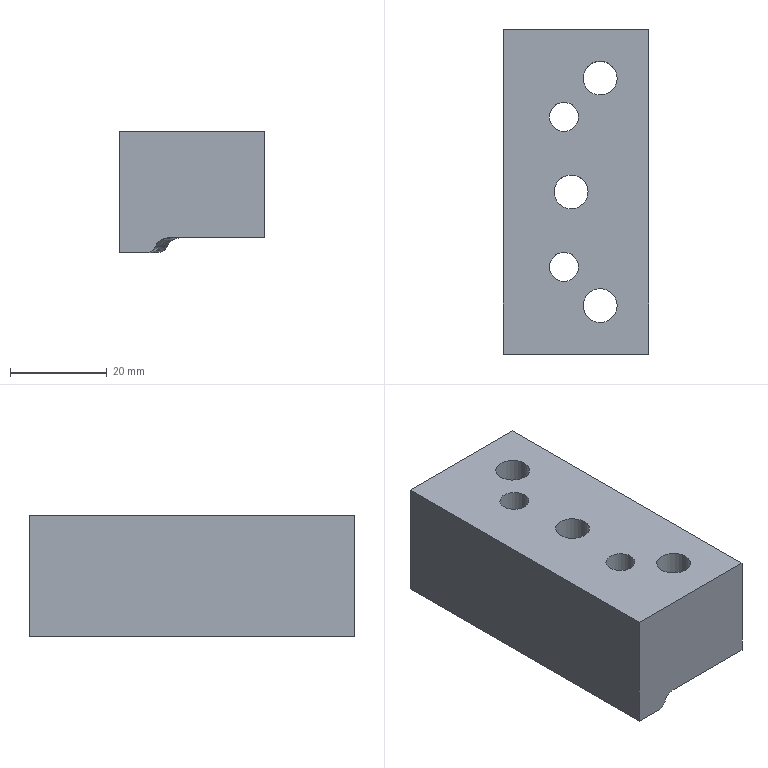Part | NX | features solid 2 | 1 solid | 24 faces | box 30 x 67 x 25 mm | volume 40202 mm3 | plane 12 | cylinder 10 | torus 2 | commonest cylinder face diameters 7 x3 11 x3 6.001 x2 6.8 x2
STEP:
#1=CARTESIAN_POINT('',(785.903,-16.315,3.));
#2=VERTEX_POINT('',#1);
#3=CARTESIAN_POINT('',(785.468,-20.349,3.));
#4=VERTEX_POINT('',#3);
#5=CARTESIAN_POINT('',(788.398,-18.625,3.));
#6=DIRECTION('',(0.,0.,1.));
#7=DIRECTION('',(1.,0.,0.));
#8=AXIS2_PLACEMENT_3D('',#5,#6,#7);
#9=CIRCLE('',#8,3.4);
#10=EDGE_CURVE('',#2,#4,#9,.T.);
#11=ORIENTED_EDGE('',*,*,#10,.F.);
#12=CARTESIAN_POINT('',(788.398,-18.625,3.));
#13=DIRECTION('',(0.,0.,1.));
#14=DIRECTION('',(1.,0.,0.));
#15=AXIS2_PLACEMENT_3D('',#12,#13,#14);
#16=CIRCLE('',#15,3.4);
#17=EDGE_CURVE('',#4,#2,#16,.T.);
#18=ORIENTED_EDGE('',*,*,#17,.F.);
#19=EDGE_LOOP('',(#11,#18));
#20=FACE_BOUND('',#19,.T.);
#21=CARTESIAN_POINT('',(791.798,-18.625,13.));
#22=VERTEX_POINT('',#21);
#23=CARTESIAN_POINT('',(788.398,-18.625,13.));
#24=DIRECTION('',(0.,0.,1.));
#25=DIRECTION('',(1.,0.,0.));
#26=AXIS2_PLACEMENT_3D('',#23,#24,#25);
#27=CIRCLE('',#26,3.4);
#28=EDGE_CURVE('',#22,#22,#27,.T.);
#29=ORIENTED_EDGE('',*,*,#28,.T.);
#30=EDGE_LOOP('',(#29));
#31=FACE_BOUND('',#30,.T.);
#32=CARTESIAN_POINT('',(788.398,-18.625,10.));
#33=DIRECTION('',(0.,0.,-1.));
#34=DIRECTION('',(1.,0.,0.));
#35=AXIS2_PLACEMENT_3D('',#32,#33,#34);
#36=CYLINDRICAL_SURFACE('',#35,3.4);
#37=ADVANCED_FACE('',(#20,#31),#36,.F.);
#38=ORIENTED_EDGE('',*,*,#28,.F.);
#39=EDGE_LOOP('',(#38));
#40=FACE_BOUND('',#39,.T.);
#41=CARTESIAN_POINT('',(791.398,-18.625,13.));
#42=VERTEX_POINT('',#41);
#43=CARTESIAN_POINT('',(788.398,-18.625,13.));
#44=DIRECTION('',(0.,0.,1.));
#45=DIRECTION('',(1.,0.,0.));
#46=AXIS2_PLACEMENT_3D('',#43,#44,#45);
#47=CIRCLE('',#46,3.001);
#48=EDGE_CURVE('',#42,#42,#47,.F.);
#49=ORIENTED_EDGE('',*,*,#48,.F.);
#50=EDGE_LOOP('',(#49));
#51=FACE_BOUND('',#50,.T.);
#52=CARTESIAN_POINT('',(788.398,-18.625,13.));
#53=DIRECTION('',(0.,0.,1.));
#54=DIRECTION('',(1.,0.,0.));
#55=AXIS2_PLACEMENT_3D('',#52,#53,#54);
#56=PLANE('',#55);
#57=ADVANCED_FACE('',(#40,#51),#56,.F.);
#58=CARTESIAN_POINT('',(792.398,-26.625,12.));
#59=VERTEX_POINT('',#58);
#60=CARTESIAN_POINT('',(795.898,-26.625,12.));
#61=DIRECTION('',(0.,0.,1.));
#62=DIRECTION('',(-1.,0.,0.));
#63=AXIS2_PLACEMENT_3D('',#60,#61,#62);
#64=CIRCLE('',#63,3.5);
#65=EDGE_CURVE('',#59,#59,#64,.F.);
#66=ORIENTED_EDGE('',*,*,#65,.F.);
#67=EDGE_LOOP('',(#66));
#68=FACE_BOUND('',#67,.T.);
#69=CARTESIAN_POINT('',(801.398,-26.625,12.));
#70=VERTEX_POINT('',#69);
#71=CARTESIAN_POINT('',(795.898,-26.625,12.));
#72=DIRECTION('',(0.,0.,-1.));
#73=DIRECTION('',(1.,0.,0.));
#74=AXIS2_PLACEMENT_3D('',#71,#72,#73);
#75=CIRCLE('',#74,5.5);
#76=EDGE_CURVE('',#70,#70,#75,.T.);
#77=ORIENTED_EDGE('',*,*,#76,.T.);
#78=EDGE_LOOP('',(#77));
#79=FACE_BOUND('',#78,.T.);
#80=CARTESIAN_POINT('',(796.378,-26.625,12.));
#81=DIRECTION('',(0.,0.,1.));
#82=DIRECTION('',(-1.,0.,0.));
#83=AXIS2_PLACEMENT_3D('',#80,#81,#82);
#84=PLANE('',#83);
#85=ADVANCED_FACE('',(#68,#79),#84,.F.);
#86=CARTESIAN_POINT('',(786.398,-3.125,12.));
#87=VERTEX_POINT('',#86);
#88=CARTESIAN_POINT('',(789.898,-3.125,12.));
#89=DIRECTION('',(0.,0.,1.));
#90=DIRECTION('',(-1.,0.,0.));
#91=AXIS2_PLACEMENT_3D('',#88,#89,#90);
#92=CIRCLE('',#91,3.5);
#93=EDGE_CURVE('',#87,#87,#92,.F.);
#94=ORIENTED_EDGE('',*,*,#93,.F.);
#95=EDGE_LOOP('',(#94));
#96=FACE_BOUND('',#95,.T.);
#97=CARTESIAN_POINT('',(795.398,-3.125,12.));
#98=VERTEX_POINT('',#97);
#99=CARTESIAN_POINT('',(789.898,-3.125,12.));
#100=DIRECTION('',(0.,0.,-1.));
#101=DIRECTION('',(1.,0.,0.));
#102=AXIS2_PLACEMENT_3D('',#99,#100,#101);
#103=CIRCLE('',#102,5.5);
#104=EDGE_CURVE('',#98,#98,#103,.T.);
#105=ORIENTED_EDGE('',*,*,#104,.T.);
#106=EDGE_LOOP('',(#105));
#107=FACE_BOUND('',#106,.T.);
#108=CARTESIAN_POINT('',(790.378,-3.125,12.));
#109=DIRECTION('',(0.,0.,1.));
#110=DIRECTION('',(-1.,0.,0.));
#111=AXIS2_PLACEMENT_3D('',#108,#109,#110);
#112=PLANE('',#111);
#113=ADVANCED_FACE('',(#96,#107),#112,.F.);
#114=CARTESIAN_POINT('',(781.518,-36.625,0.));
#115=VERTEX_POINT('',#114);
#116=CARTESIAN_POINT('',(783.985,30.375,0.));
#117=VERTEX_POINT('',#116);
#118=CARTESIAN_POINT('',(1009.499,-11.474,0.));
#119=DIRECTION('',(0.,0.,1.));
#120=DIRECTION('',(1.,0.,0.));
#121=AXIS2_PLACEMENT_3D('',#118,#119,#120);
#122=CIRCLE('',#121,229.364);
#123=EDGE_CURVE('',#115,#117,#122,.F.);
#124=ORIENTED_EDGE('',*,*,#123,.F.);
#125=CARTESIAN_POINT('',(775.898,-36.625,0.));
#126=VERTEX_POINT('',#125);
#127=CARTESIAN_POINT('',(795.878,-36.625,0.));
#128=DIRECTION('',(-1.,0.,0.));
#129=VECTOR('',#128,1000.);
#130=LINE('',#127,#129);
#131=EDGE_CURVE('',#115,#126,#130,.T.);
#132=ORIENTED_EDGE('',*,*,#131,.T.);
#133=CARTESIAN_POINT('',(775.898,30.375,0.));
#134=VERTEX_POINT('',#133);
#135=CARTESIAN_POINT('',(775.898,0.7578,0.));
#136=DIRECTION('',(0.,-1.,0.));
#137=VECTOR('',#136,1000.);
#138=LINE('',#135,#137);
#139=EDGE_CURVE('',#134,#126,#138,.T.);
#140=ORIENTED_EDGE('',*,*,#139,.F.);
#141=CARTESIAN_POINT('',(795.878,30.375,0.));
#142=DIRECTION('',(-1.,0.,0.));
#143=VECTOR('',#142,1000.);
#144=LINE('',#141,#143);
#145=EDGE_CURVE('',#117,#134,#144,.T.);
#146=ORIENTED_EDGE('',*,*,#145,.F.);
#147=EDGE_LOOP('',(#124,#132,#140,#146));
#148=FACE_BOUND('',#147,.T.);
#149=CARTESIAN_POINT('',(445.33,343.366,0.));
#150=DIRECTION('',(0.,0.,1.));
#151=DIRECTION('',(0.,-1.,0.));
#152=AXIS2_PLACEMENT_3D('',#149,#150,#151);
#153=PLANE('',#152);
#154=ADVANCED_FACE('',(#148),#153,.F.);
#155=CARTESIAN_POINT('',(791.798,12.375,13.));
#156=VERTEX_POINT('',#155);
#157=CARTESIAN_POINT('',(788.398,12.375,13.));
#158=DIRECTION('',(0.,0.,1.));
#159=DIRECTION('',(1.,0.,0.));
#160=AXIS2_PLACEMENT_3D('',#157,#158,#159);
#161=CIRCLE('',#160,3.4);
#162=EDGE_CURVE('',#156,#156,#161,.T.);
#163=ORIENTED_EDGE('',*,*,#162,.F.);
#164=EDGE_LOOP('',(#163));
#165=FACE_BOUND('',#164,.T.);
#166=CARTESIAN_POINT('',(791.398,12.375,13.));
#167=VERTEX_POINT('',#166);
#168=CARTESIAN_POINT('',(788.398,12.375,13.));
#169=DIRECTION('',(0.,0.,1.));
#170=DIRECTION('',(1.,0.,0.));
#171=AXIS2_PLACEMENT_3D('',#168,#169,#170);
#172=CIRCLE('',#171,3.001);
#173=EDGE_CURVE('',#167,#167,#172,.F.);
#174=ORIENTED_EDGE('',*,*,#173,.F.);
#175=EDGE_LOOP('',(#174));
#176=FACE_BOUND('',#175,.T.);
#177=CARTESIAN_POINT('',(788.398,12.375,13.));
#178=DIRECTION('',(0.,0.,1.));
#179=DIRECTION('',(1.,0.,0.));
#180=AXIS2_PLACEMENT_3D('',#177,#178,#179);
#181=PLANE('',#180);
#182=ADVANCED_FACE('',(#165,#176),#181,.F.);
#183=CARTESIAN_POINT('',(785.903,30.375,1.333));
#184=VERTEX_POINT('',#183);
#185=CARTESIAN_POINT('',(783.985,30.375,0.));
#186=CARTESIAN_POINT('',(784.822,30.375,0.));
#187=CARTESIAN_POINT('',(785.62,30.375,0.5458));
#188=CARTESIAN_POINT('',(785.903,30.375,1.333));
#189=B_SPLINE_CURVE_WITH_KNOTS('',3,(#185,#186,#187,#188),.UNSPECIFIED.,.F.,.F.,(4,4),(0.,0.002474),.UNSPECIFIED.);
#190=EDGE_CURVE('',#117,#184,#189,.T.);
#191=ORIENTED_EDGE('',*,*,#190,.T.);
#192=CARTESIAN_POINT('',(783.415,-36.625,1.333));
#193=VERTEX_POINT('',#192);
#194=CARTESIAN_POINT('',(1009.499,-11.474,1.333));
#195=DIRECTION('',(0.,0.,1.));
#196=DIRECTION('',(1.,0.,0.));
#197=AXIS2_PLACEMENT_3D('',#194,#195,#196);
#198=CIRCLE('',#197,227.478);
#199=EDGE_CURVE('',#193,#184,#198,.F.);
#200=ORIENTED_EDGE('',*,*,#199,.F.);
#201=CARTESIAN_POINT('',(781.518,-36.625,0.));
#202=CARTESIAN_POINT('',(782.338,-36.625,0.));
#203=CARTESIAN_POINT('',(783.139,-36.625,0.5563));
#204=CARTESIAN_POINT('',(783.415,-36.625,1.333));
#205=B_SPLINE_CURVE_WITH_KNOTS('',3,(#201,#202,#203,#204),.UNSPECIFIED.,.F.,.F.,(4,4),(0.001047,0.003506),.UNSPECIFIED.);
#206=EDGE_CURVE('',#115,#193,#205,.T.);
#207=ORIENTED_EDGE('',*,*,#206,.F.);
#208=ORIENTED_EDGE('',*,*,#123,.T.);
#209=EDGE_LOOP('',(#191,#200,#207,#208));
#210=FACE_BOUND('',#209,.T.);
#211=CARTESIAN_POINT('',(1009.499,-11.474,2.));
#212=DIRECTION('',(0.,0.,1.));
#213=DIRECTION('',(0.9656,-0.2602,0.));
#214=AXIS2_PLACEMENT_3D('',#211,#212,#213);
#215=TOROIDAL_SURFACE('',#214,229.364,2.);
#216=ADVANCED_FACE('',(#210),#215,.T.);
#217=CARTESIAN_POINT('',(792.398,20.375,12.));
#218=VERTEX_POINT('',#217);
#219=CARTESIAN_POINT('',(795.898,20.375,12.));
#220=DIRECTION('',(0.,0.,-1.));
#221=DIRECTION('',(-1.,0.,0.));
#222=AXIS2_PLACEMENT_3D('',#219,#220,#221);
#223=CIRCLE('',#222,3.5);
#224=EDGE_CURVE('',#218,#218,#223,.F.);
#225=ORIENTED_EDGE('',*,*,#224,.T.);
#226=EDGE_LOOP('',(#225));
#227=FACE_BOUND('',#226,.T.);
#228=CARTESIAN_POINT('',(801.398,20.375,12.));
#229=VERTEX_POINT('',#228);
#230=CARTESIAN_POINT('',(795.898,20.375,12.));
#231=DIRECTION('',(0.,0.,1.));
#232=DIRECTION('',(1.,0.,0.));
#233=AXIS2_PLACEMENT_3D('',#230,#231,#232);
#234=CIRCLE('',#233,5.5);
#235=EDGE_CURVE('',#229,#229,#234,.T.);
#236=ORIENTED_EDGE('',*,*,#235,.F.);
#237=EDGE_LOOP('',(#236));
#238=FACE_BOUND('',#237,.T.);
#239=CARTESIAN_POINT('',(796.378,20.375,12.));
#240=DIRECTION('',(0.,0.,1.));
#241=DIRECTION('',(-1.,0.,0.));
#242=AXIS2_PLACEMENT_3D('',#239,#240,#241);
#243=PLANE('',#242);
#244=ADVANCED_FACE('',(#227,#238),#243,.F.);
#245=ORIENTED_EDGE('',*,*,#76,.F.);
#246=EDGE_LOOP('',(#245));
#247=FACE_BOUND('',#246,.T.);
#248=CARTESIAN_POINT('',(801.398,-26.625,3.));
#249=VERTEX_POINT('',#248);
#250=CARTESIAN_POINT('',(795.898,-26.625,3.));
#251=DIRECTION('',(0.,0.,1.));
#252=DIRECTION('',(1.,0.,0.));
#253=AXIS2_PLACEMENT_3D('',#250,#251,#252);
#254=CIRCLE('',#253,5.5);
#255=EDGE_CURVE('',#249,#249,#254,.F.);
#256=ORIENTED_EDGE('',*,*,#255,.T.);
#257=EDGE_LOOP('',(#256));
#258=FACE_BOUND('',#257,.T.);
#259=CARTESIAN_POINT('',(795.898,-26.625,3.));
#260=DIRECTION('',(0.,0.,1.));
#261=DIRECTION('',(1.,0.,0.));
#262=AXIS2_PLACEMENT_3D('',#259,#260,#261);
#263=CYLINDRICAL_SURFACE('',#262,5.5);
#264=ADVANCED_FACE('',(#247,#258),#263,.F.);
#265=ORIENTED_EDGE('',*,*,#104,.F.);
#266=EDGE_LOOP('',(#265));
#267=FACE_BOUND('',#266,.T.);
#268=CARTESIAN_POINT('',(784.591,-1.68,3.));
#269=VERTEX_POINT('',#268);
#270=CARTESIAN_POINT('',(784.496,-4.163,3.));
#271=VERTEX_POINT('',#270);
#272=CARTESIAN_POINT('',(789.898,-3.125,3.));
#273=DIRECTION('',(0.,0.,1.));
#274=DIRECTION('',(1.,0.,0.));
#275=AXIS2_PLACEMENT_3D('',#272,#273,#274);
#276=CIRCLE('',#275,5.5);
#277=EDGE_CURVE('',#269,#271,#276,.F.);
#278=ORIENTED_EDGE('',*,*,#277,.T.);
#279=CARTESIAN_POINT('',(784.591,-1.68,3.));
#280=CARTESIAN_POINT('',(784.371,-2.487,3.));
#281=CARTESIAN_POINT('',(784.339,-3.345,3.));
#282=CARTESIAN_POINT('',(784.496,-4.163,3.));
#283=B_SPLINE_CURVE_WITH_KNOTS('',3,(#279,#280,#281,#282),.UNSPECIFIED.,.F.,.F.,(4,4),(0.005013,0.007519),.UNSPECIFIED.);
#284=EDGE_CURVE('',#269,#271,#283,.T.);
#285=ORIENTED_EDGE('',*,*,#284,.F.);
#286=EDGE_LOOP('',(#278,#285));
#287=FACE_BOUND('',#286,.T.);
#288=CARTESIAN_POINT('',(789.898,-3.125,3.));
#289=DIRECTION('',(0.,0.,1.));
#290=DIRECTION('',(1.,0.,0.));
#291=AXIS2_PLACEMENT_3D('',#288,#289,#290);
#292=CYLINDRICAL_SURFACE('',#291,5.5);
#293=ADVANCED_FACE('',(#267,#287),#292,.F.);
#294=CARTESIAN_POINT('',(805.898,-36.625,3.));
#295=VERTEX_POINT('',#294);
#296=CARTESIAN_POINT('',(785.787,-36.625,3.));
#297=VERTEX_POINT('',#296);
#298=CARTESIAN_POINT('',(795.878,-36.625,3.));
#299=DIRECTION('',(-1.,0.,0.));
#300=VECTOR('',#299,1000.);
#301=LINE('',#298,#300);
#302=EDGE_CURVE('',#295,#297,#301,.T.);
#303=ORIENTED_EDGE('',*,*,#302,.F.);
#304=CARTESIAN_POINT('',(805.898,-36.625,25.));
#305=VERTEX_POINT('',#304);
#306=CARTESIAN_POINT('',(805.898,-36.625,20.));
#307=DIRECTION('',(0.,0.,1.));
#308=VECTOR('',#307,1000.);
#309=LINE('',#306,#308);
#310=EDGE_CURVE('',#295,#305,#309,.T.);
#311=ORIENTED_EDGE('',*,*,#310,.T.);
#312=CARTESIAN_POINT('',(775.898,-36.625,25.));
#313=VERTEX_POINT('',#312);
#314=CARTESIAN_POINT('',(512.,-36.625,25.));
#315=DIRECTION('',(-1.,0.,0.));
#316=VECTOR('',#315,1000.);
#317=LINE('',#314,#316);
#318=EDGE_CURVE('',#305,#313,#317,.T.);
#319=ORIENTED_EDGE('',*,*,#318,.T.);
#320=CARTESIAN_POINT('',(775.898,-36.625,20.));
#321=DIRECTION('',(0.,0.,1.));
#322=VECTOR('',#321,1000.);
#323=LINE('',#320,#322);
#324=EDGE_CURVE('',#126,#313,#323,.T.);
#325=ORIENTED_EDGE('',*,*,#324,.F.);
#326=ORIENTED_EDGE('',*,*,#131,.F.);
#327=ORIENTED_EDGE('',*,*,#206,.T.);
#328=CARTESIAN_POINT('',(785.787,-36.625,3.));
#329=CARTESIAN_POINT('',(784.763,-36.625,3.));
#330=CARTESIAN_POINT('',(783.759,-36.625,2.298));
#331=CARTESIAN_POINT('',(783.415,-36.625,1.333));
#332=B_SPLINE_CURVE_WITH_KNOTS('',3,(#328,#329,#330,#331),.UNSPECIFIED.,.F.,.F.,(4,4),(0.01298,0.01605),.UNSPECIFIED.);
#333=EDGE_CURVE('',#297,#193,#332,.T.);
#334=ORIENTED_EDGE('',*,*,#333,.F.);
#335=EDGE_LOOP('',(#303,#311,#319,#325,#326,#327,#334));
#336=FACE_BOUND('',#335,.T.);
#337=CARTESIAN_POINT('',(795.878,-36.625,20.));
#338=DIRECTION('',(0.,-1.,0.));
#339=DIRECTION('',(0.,0.,-1.));
#340=AXIS2_PLACEMENT_3D('',#337,#338,#339);
#341=PLANE('',#340);
#342=ADVANCED_FACE('',(#336),#341,.T.);
#343=CARTESIAN_POINT('',(805.898,30.375,3.));
#344=VERTEX_POINT('',#343);
#345=CARTESIAN_POINT('',(805.898,0.7578,3.));
#346=DIRECTION('',(0.,-1.,0.));
#347=VECTOR('',#346,1000.);
#348=LINE('',#345,#347);
#349=EDGE_CURVE('',#344,#295,#348,.T.);
#350=ORIENTED_EDGE('',*,*,#349,.F.);
#351=CARTESIAN_POINT('',(805.898,30.375,25.));
#352=VERTEX_POINT('',#351);
#353=CARTESIAN_POINT('',(805.898,30.375,0.));
#354=DIRECTION('',(0.,0.,1.));
#355=VECTOR('',#354,1000.);
#356=LINE('',#353,#355);
#357=EDGE_CURVE('',#344,#352,#356,.T.);
#358=ORIENTED_EDGE('',*,*,#357,.T.);
#359=CARTESIAN_POINT('',(805.898,0.,25.));
#360=DIRECTION('',(0.,-1.,0.));
#361=VECTOR('',#360,1000.);
#362=LINE('',#359,#361);
#363=EDGE_CURVE('',#352,#305,#362,.T.);
#364=ORIENTED_EDGE('',*,*,#363,.T.);
#365=ORIENTED_EDGE('',*,*,#310,.F.);
#366=EDGE_LOOP('',(#350,#358,#364,#365));
#367=FACE_BOUND('',#366,.T.);
#368=CARTESIAN_POINT('',(805.898,0.7578,0.));
#369=DIRECTION('',(1.,0.,0.));
#370=DIRECTION('',(0.,0.,-1.));
#371=AXIS2_PLACEMENT_3D('',#368,#369,#370);
#372=PLANE('',#371);
#373=ADVANCED_FACE('',(#367),#372,.T.);
#374=ORIENTED_EDGE('',*,*,#357,.F.);
#375=CARTESIAN_POINT('',(788.302,30.375,3.));
#376=VERTEX_POINT('',#375);
#377=CARTESIAN_POINT('',(795.878,30.375,3.));
#378=DIRECTION('',(-1.,0.,0.));
#379=VECTOR('',#378,1000.);
#380=LINE('',#377,#379);
#381=EDGE_CURVE('',#344,#376,#380,.T.);
#382=ORIENTED_EDGE('',*,*,#381,.T.);
#383=CARTESIAN_POINT('',(788.302,30.375,3.));
#384=CARTESIAN_POINT('',(787.256,30.375,3.));
#385=CARTESIAN_POINT('',(786.258,30.375,2.318));
#386=CARTESIAN_POINT('',(785.903,30.375,1.333));
#387=B_SPLINE_CURVE_WITH_KNOTS('',3,(#383,#384,#385,#386),.UNSPECIFIED.,.F.,.F.,(4,4),(0.,0.003094),.UNSPECIFIED.);
#388=EDGE_CURVE('',#376,#184,#387,.T.);
#389=ORIENTED_EDGE('',*,*,#388,.T.);
#390=ORIENTED_EDGE('',*,*,#190,.F.);
#391=ORIENTED_EDGE('',*,*,#145,.T.);
#392=CARTESIAN_POINT('',(775.898,30.375,25.));
#393=VERTEX_POINT('',#392);
#394=CARTESIAN_POINT('',(775.898,30.375,0.));
#395=DIRECTION('',(0.,0.,1.));
#396=VECTOR('',#395,1000.);
#397=LINE('',#394,#396);
#398=EDGE_CURVE('',#134,#393,#397,.T.);
#399=ORIENTED_EDGE('',*,*,#398,.T.);
#400=CARTESIAN_POINT('',(512.,30.375,25.));
#401=DIRECTION('',(-1.,0.,0.));
#402=VECTOR('',#401,1000.);
#403=LINE('',#400,#402);
#404=EDGE_CURVE('',#352,#393,#403,.T.);
#405=ORIENTED_EDGE('',*,*,#404,.F.);
#406=EDGE_LOOP('',(#374,#382,#389,#390,#391,#399,#405));
#407=FACE_BOUND('',#406,.T.);
#408=CARTESIAN_POINT('',(795.878,30.375,0.));
#409=DIRECTION('',(0.,-1.,0.));
#410=DIRECTION('',(0.,0.,-1.));
#411=AXIS2_PLACEMENT_3D('',#408,#409,#410);
#412=PLANE('',#411);
#413=ADVANCED_FACE('',(#407),#412,.F.);
#414=ORIENTED_EDGE('',*,*,#162,.T.);
#415=EDGE_LOOP('',(#414));
#416=FACE_BOUND('',#415,.T.);
#417=CARTESIAN_POINT('',(785.903,14.685,3.));
#418=VERTEX_POINT('',#417);
#419=CARTESIAN_POINT('',(785.468,10.651,3.));
#420=VERTEX_POINT('',#419);
#421=CARTESIAN_POINT('',(785.903,14.685,3.));
#422=CARTESIAN_POINT('',(785.409,14.151,3.));
#423=CARTESIAN_POINT('',(784.779,12.764,2.821));
#424=CARTESIAN_POINT('',(785.101,11.273,3.));
#425=CARTESIAN_POINT('',(785.468,10.651,3.));
#426=B_SPLINE_CURVE_WITH_KNOTS('',3,(#421,#422,#423,#424,#425),.UNSPECIFIED.,.F.,.F.,(4,1,4),(0.003221,0.005391,0.007562),.UNSPECIFIED.);
#427=EDGE_CURVE('',#418,#420,#426,.T.);
#428=ORIENTED_EDGE('',*,*,#427,.F.);
#429=CARTESIAN_POINT('',(788.398,12.375,3.));
#430=DIRECTION('',(0.,0.,1.));
#431=DIRECTION('',(1.,0.,0.));
#432=AXIS2_PLACEMENT_3D('',#429,#430,#431);
#433=CIRCLE('',#432,3.4);
#434=EDGE_CURVE('',#420,#418,#433,.T.);
#435=ORIENTED_EDGE('',*,*,#434,.F.);
#436=EDGE_LOOP('',(#428,#435));
#437=FACE_BOUND('',#436,.T.);
#438=CARTESIAN_POINT('',(788.398,12.375,10.));
#439=DIRECTION('',(0.,0.,-1.));
#440=DIRECTION('',(1.,0.,0.));
#441=AXIS2_PLACEMENT_3D('',#438,#439,#440);
#442=CYLINDRICAL_SURFACE('',#441,3.4);
#443=ADVANCED_FACE('',(#416,#437),#442,.F.);
#444=CARTESIAN_POINT('',(1009.499,-11.474,3.));
#445=DIRECTION('',(0.,0.,1.));
#446=DIRECTION('',(1.,0.,0.));
#447=AXIS2_PLACEMENT_3D('',#444,#445,#446);
#448=CIRCLE('',#447,225.121);
#449=EDGE_CURVE('',#418,#376,#448,.F.);
#450=ORIENTED_EDGE('',*,*,#449,.F.);
#451=ORIENTED_EDGE('',*,*,#427,.T.);
#452=CARTESIAN_POINT('',(1009.499,-11.474,3.));
#453=DIRECTION('',(0.,0.,1.));
#454=DIRECTION('',(1.,0.,0.));
#455=AXIS2_PLACEMENT_3D('',#452,#453,#454);
#456=CIRCLE('',#455,225.121);
#457=EDGE_CURVE('',#269,#420,#456,.F.);
#458=ORIENTED_EDGE('',*,*,#457,.F.);
#459=ORIENTED_EDGE('',*,*,#284,.T.);
#460=CARTESIAN_POINT('',(1009.499,-11.474,3.));
#461=DIRECTION('',(0.,0.,1.));
#462=DIRECTION('',(1.,0.,0.));
#463=AXIS2_PLACEMENT_3D('',#460,#461,#462);
#464=CIRCLE('',#463,225.121);
#465=EDGE_CURVE('',#297,#271,#464,.F.);
#466=ORIENTED_EDGE('',*,*,#465,.F.);
#467=ORIENTED_EDGE('',*,*,#333,.T.);
#468=ORIENTED_EDGE('',*,*,#199,.T.);
#469=ORIENTED_EDGE('',*,*,#388,.F.);
#470=EDGE_LOOP('',(#450,#451,#458,#459,#466,#467,#468,#469));
#471=FACE_BOUND('',#470,.T.);
#472=CARTESIAN_POINT('',(1009.499,-11.474,0.5));
#473=DIRECTION('',(0.,0.,1.));
#474=DIRECTION('',(0.9656,-0.2602,0.));
#475=AXIS2_PLACEMENT_3D('',#472,#473,#474);
#476=TOROIDAL_SURFACE('',#475,225.121,2.5);
#477=ADVANCED_FACE('',(#471),#476,.F.);
#478=ORIENTED_EDGE('',*,*,#235,.T.);
#479=EDGE_LOOP('',(#478));
#480=FACE_BOUND('',#479,.T.);
#481=CARTESIAN_POINT('',(801.398,20.375,3.));
#482=VERTEX_POINT('',#481);
#483=CARTESIAN_POINT('',(795.898,20.375,3.));
#484=DIRECTION('',(0.,0.,-1.));
#485=DIRECTION('',(1.,0.,0.));
#486=AXIS2_PLACEMENT_3D('',#483,#484,#485);
#487=CIRCLE('',#486,5.5);
#488=EDGE_CURVE('',#482,#482,#487,.F.);
#489=ORIENTED_EDGE('',*,*,#488,.F.);
#490=EDGE_LOOP('',(#489));
#491=FACE_BOUND('',#490,.T.);
#492=CARTESIAN_POINT('',(795.898,20.375,3.));
#493=DIRECTION('',(0.,0.,1.));
#494=DIRECTION('',(1.,0.,0.));
#495=AXIS2_PLACEMENT_3D('',#492,#493,#494);
#496=CYLINDRICAL_SURFACE('',#495,5.5);
#497=ADVANCED_FACE('',(#480,#491),#496,.F.);
#498=ORIENTED_EDGE('',*,*,#17,.T.);
#499=ORIENTED_EDGE('',*,*,#10,.T.);
#500=EDGE_LOOP('',(#498,#499));
#501=FACE_BOUND('',#500,.T.);
#502=ORIENTED_EDGE('',*,*,#488,.T.);
#503=EDGE_LOOP('',(#502));
#504=FACE_BOUND('',#503,.T.);
#505=ORIENTED_EDGE('',*,*,#457,.T.);
#506=ORIENTED_EDGE('',*,*,#434,.T.);
#507=ORIENTED_EDGE('',*,*,#449,.T.);
#508=ORIENTED_EDGE('',*,*,#381,.F.);
#509=ORIENTED_EDGE('',*,*,#349,.T.);
#510=ORIENTED_EDGE('',*,*,#302,.T.);
#511=ORIENTED_EDGE('',*,*,#465,.T.);
#512=ORIENTED_EDGE('',*,*,#277,.F.);
#513=EDGE_LOOP('',(#505,#506,#507,#508,#509,#510,#511,#512));
#514=FACE_BOUND('',#513,.T.);
#515=ORIENTED_EDGE('',*,*,#255,.F.);
#516=EDGE_LOOP('',(#515));
#517=FACE_BOUND('',#516,.T.);
#518=CARTESIAN_POINT('',(445.33,343.366,3.));
#519=DIRECTION('',(0.,0.,1.));
#520=DIRECTION('',(0.,-1.,0.));
#521=AXIS2_PLACEMENT_3D('',#518,#519,#520);
#522=PLANE('',#521);
#523=ADVANCED_FACE('',(#501,#504,#514,#517),#522,.F.);
#524=ORIENTED_EDGE('',*,*,#398,.F.);
#525=ORIENTED_EDGE('',*,*,#139,.T.);
#526=ORIENTED_EDGE('',*,*,#324,.T.);
#527=CARTESIAN_POINT('',(775.898,0.,25.));
#528=DIRECTION('',(0.,-1.,0.));
#529=VECTOR('',#528,1000.);
#530=LINE('',#527,#529);
#531=EDGE_CURVE('',#393,#313,#530,.T.);
#532=ORIENTED_EDGE('',*,*,#531,.F.);
#533=EDGE_LOOP('',(#524,#525,#526,#532));
#534=FACE_BOUND('',#533,.T.);
#535=CARTESIAN_POINT('',(775.898,0.7578,0.));
#536=DIRECTION('',(1.,0.,0.));
#537=DIRECTION('',(0.,0.,-1.));
#538=AXIS2_PLACEMENT_3D('',#535,#536,#537);
#539=PLANE('',#538);
#540=ADVANCED_FACE('',(#534),#539,.F.);
#541=ORIENTED_EDGE('',*,*,#93,.T.);
#542=EDGE_LOOP('',(#541));
#543=FACE_BOUND('',#542,.T.);
#544=CARTESIAN_POINT('',(786.398,-3.125,25.));
#545=VERTEX_POINT('',#544);
#546=CARTESIAN_POINT('',(789.898,-3.125,25.));
#547=DIRECTION('',(0.,0.,-1.));
#548=DIRECTION('',(-1.,0.,0.));
#549=AXIS2_PLACEMENT_3D('',#546,#547,#548);
#550=CIRCLE('',#549,3.5);
#551=EDGE_CURVE('',#545,#545,#550,.T.);
#552=ORIENTED_EDGE('',*,*,#551,.F.);
#553=EDGE_LOOP('',(#552));
#554=FACE_BOUND('',#553,.T.);
#555=CARTESIAN_POINT('',(789.898,-3.125,1.));
#556=DIRECTION('',(0.,0.,1.));
#557=DIRECTION('',(1.,0.,0.));
#558=AXIS2_PLACEMENT_3D('',#555,#556,#557);
#559=CYLINDRICAL_SURFACE('',#558,3.5);
#560=ADVANCED_FACE('',(#543,#554),#559,.F.);
#561=ORIENTED_EDGE('',*,*,#65,.T.);
#562=EDGE_LOOP('',(#561));
#563=FACE_BOUND('',#562,.T.);
#564=CARTESIAN_POINT('',(792.398,-26.625,25.));
#565=VERTEX_POINT('',#564);
#566=CARTESIAN_POINT('',(795.898,-26.625,25.));
#567=DIRECTION('',(0.,0.,-1.));
#568=DIRECTION('',(-1.,0.,0.));
#569=AXIS2_PLACEMENT_3D('',#566,#567,#568);
#570=CIRCLE('',#569,3.5);
#571=EDGE_CURVE('',#565,#565,#570,.T.);
#572=ORIENTED_EDGE('',*,*,#571,.F.);
#573=EDGE_LOOP('',(#572));
#574=FACE_BOUND('',#573,.T.);
#575=CARTESIAN_POINT('',(795.898,-26.625,1.));
#576=DIRECTION('',(0.,0.,1.));
#577=DIRECTION('',(1.,0.,0.));
#578=AXIS2_PLACEMENT_3D('',#575,#576,#577);
#579=CYLINDRICAL_SURFACE('',#578,3.5);
#580=ADVANCED_FACE('',(#563,#574),#579,.F.);
#581=ORIENTED_EDGE('',*,*,#173,.T.);
#582=EDGE_LOOP('',(#581));
#583=FACE_BOUND('',#582,.T.);
#584=CARTESIAN_POINT('',(785.397,12.375,25.));
#585=VERTEX_POINT('',#584);
#586=CARTESIAN_POINT('',(788.398,12.375,25.));
#587=DIRECTION('',(0.,0.,-1.));
#588=DIRECTION('',(-1.,0.,0.));
#589=AXIS2_PLACEMENT_3D('',#586,#587,#588);
#590=CIRCLE('',#589,3.001);
#591=EDGE_CURVE('',#585,#585,#590,.T.);
#592=ORIENTED_EDGE('',*,*,#591,.F.);
#593=EDGE_LOOP('',(#592));
#594=FACE_BOUND('',#593,.T.);
#595=CARTESIAN_POINT('',(788.398,12.375,1.));
#596=DIRECTION('',(0.,0.,1.));
#597=DIRECTION('',(1.,0.,0.));
#598=AXIS2_PLACEMENT_3D('',#595,#596,#597);
#599=CYLINDRICAL_SURFACE('',#598,3.001);
#600=ADVANCED_FACE('',(#583,#594),#599,.F.);
#601=ORIENTED_EDGE('',*,*,#224,.F.);
#602=EDGE_LOOP('',(#601));
#603=FACE_BOUND('',#602,.T.);
#604=CARTESIAN_POINT('',(792.398,20.375,25.));
#605=VERTEX_POINT('',#604);
#606=CARTESIAN_POINT('',(795.898,20.375,25.));
#607=DIRECTION('',(0.,0.,-1.));
#608=DIRECTION('',(-1.,0.,0.));
#609=AXIS2_PLACEMENT_3D('',#606,#607,#608);
#610=CIRCLE('',#609,3.5);
#611=EDGE_CURVE('',#605,#605,#610,.T.);
#612=ORIENTED_EDGE('',*,*,#611,.F.);
#613=EDGE_LOOP('',(#612));
#614=FACE_BOUND('',#613,.T.);
#615=CARTESIAN_POINT('',(795.898,20.375,1.));
#616=DIRECTION('',(0.,0.,1.));
#617=DIRECTION('',(1.,0.,0.));
#618=AXIS2_PLACEMENT_3D('',#615,#616,#617);
#619=CYLINDRICAL_SURFACE('',#618,3.5);
#620=ADVANCED_FACE('',(#603,#614),#619,.F.);
#621=ORIENTED_EDGE('',*,*,#611,.T.);
#622=EDGE_LOOP('',(#621));
#623=FACE_BOUND('',#622,.T.);
#624=ORIENTED_EDGE('',*,*,#591,.T.);
#625=EDGE_LOOP('',(#624));
#626=FACE_BOUND('',#625,.T.);
#627=CARTESIAN_POINT('',(785.397,-18.625,25.));
#628=VERTEX_POINT('',#627);
#629=CARTESIAN_POINT('',(788.398,-18.625,25.));
#630=DIRECTION('',(0.,0.,-1.));
#631=DIRECTION('',(-1.,0.,0.));
#632=AXIS2_PLACEMENT_3D('',#629,#630,#631);
#633=CIRCLE('',#632,3.001);
#634=EDGE_CURVE('',#628,#628,#633,.T.);
#635=ORIENTED_EDGE('',*,*,#634,.T.);
#636=EDGE_LOOP('',(#635));
#637=FACE_BOUND('',#636,.T.);
#638=ORIENTED_EDGE('',*,*,#571,.T.);
#639=EDGE_LOOP('',(#638));
#640=FACE_BOUND('',#639,.T.);
#641=ORIENTED_EDGE('',*,*,#551,.T.);
#642=EDGE_LOOP('',(#641));
#643=FACE_BOUND('',#642,.T.);
#644=ORIENTED_EDGE('',*,*,#531,.T.);
#645=ORIENTED_EDGE('',*,*,#318,.F.);
#646=ORIENTED_EDGE('',*,*,#363,.F.);
#647=ORIENTED_EDGE('',*,*,#404,.T.);
#648=EDGE_LOOP('',(#644,#645,#646,#647));
#649=FACE_BOUND('',#648,.T.);
#650=CARTESIAN_POINT('',(512.,0.,25.));
#651=DIRECTION('',(0.,0.,-1.));
#652=DIRECTION('',(-1.,0.,0.));
#653=AXIS2_PLACEMENT_3D('',#650,#651,#652);
#654=PLANE('',#653);
#655=ADVANCED_FACE('',(#623,#626,#637,#640,#643,#649),#654,.F.);
#656=ORIENTED_EDGE('',*,*,#48,.T.);
#657=EDGE_LOOP('',(#656));
#658=FACE_BOUND('',#657,.T.);
#659=ORIENTED_EDGE('',*,*,#634,.F.);
#660=EDGE_LOOP('',(#659));
#661=FACE_BOUND('',#660,.T.);
#662=CARTESIAN_POINT('',(788.398,-18.625,1.));
#663=DIRECTION('',(0.,0.,1.));
#664=DIRECTION('',(1.,0.,0.));
#665=AXIS2_PLACEMENT_3D('',#662,#663,#664);
#666=CYLINDRICAL_SURFACE('',#665,3.001);
#667=ADVANCED_FACE('',(#658,#661),#666,.F.);
#668=CLOSED_SHELL('',(#37,#57,#85,#113,#154,#182,#216,#244,#264,#293,#342,#373,#413,#443,#477,#497,#523,#540,#560,#580,#600,#620,#655,#667));
#669=MANIFOLD_SOLID_BREP('',#668);
#670=(LENGTH_UNIT()NAMED_UNIT(*)SI_UNIT(.MILLI.,.METRE.));
#671=UNCERTAINTY_MEASURE_WITH_UNIT(LENGTH_MEASURE(0.0508),#670,'','');
#672=(NAMED_UNIT(*)PLANE_ANGLE_UNIT()SI_UNIT($,.RADIAN.));
#673=(NAMED_UNIT(*)SI_UNIT($,.STERADIAN.)SOLID_ANGLE_UNIT());
#674=(GEOMETRIC_REPRESENTATION_CONTEXT(3)GLOBAL_UNCERTAINTY_ASSIGNED_CONTEXT((#671))GLOBAL_UNIT_ASSIGNED_CONTEXT((#670,#672,#673))REPRESENTATION_CONTEXT('',''));
#675=ADVANCED_BREP_SHAPE_REPRESENTATION('',(#669),#674);